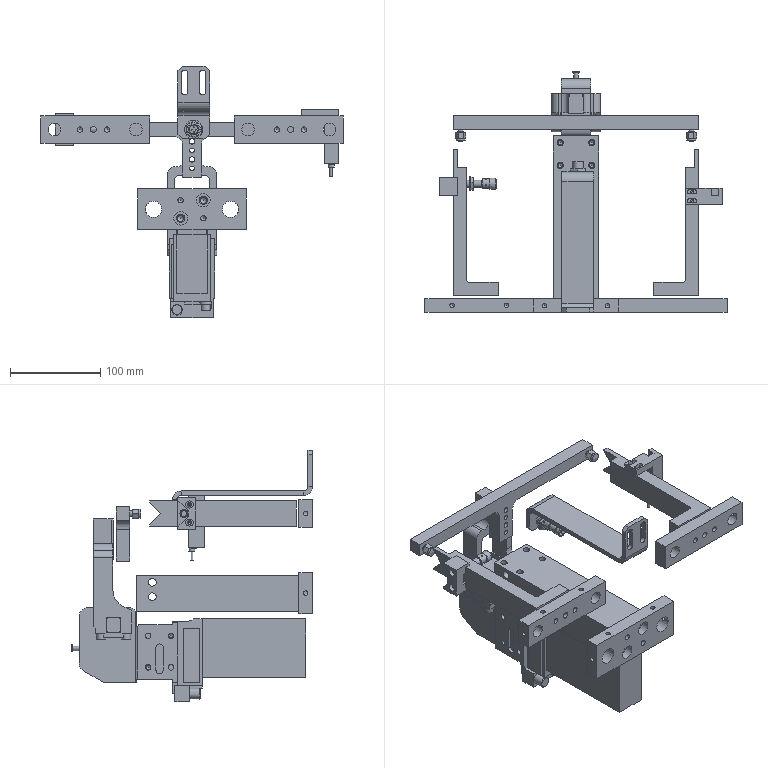Part | NX | features BREP 24 | 30 solids | 878 faces | box 333.8 x 266.25 x 278 mm | volume 1517333 mm3 | plane 490 | cylinder 286 | cone 100 | sphere 2 | commonest cylinder face diameters 6 x31 15 x30 13 x22 1.875 x20 1 x16 5 x16